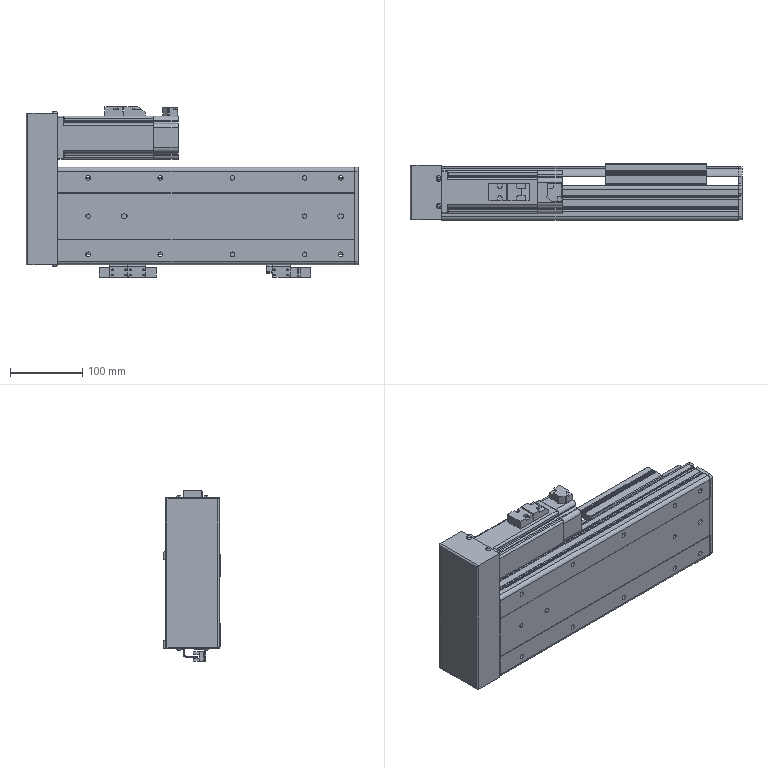Part | SolidWorks | 12 solids | 766 faces | box 460 x 78 x 235.85 mm | volume 3440489 mm3 | plane 400 | cylinder 312 | cone 46 | torus 8 | commonest cylinder face diameters 6 x37 2 x36 1 x30 2.5 x24 6.647 x20 11 x20